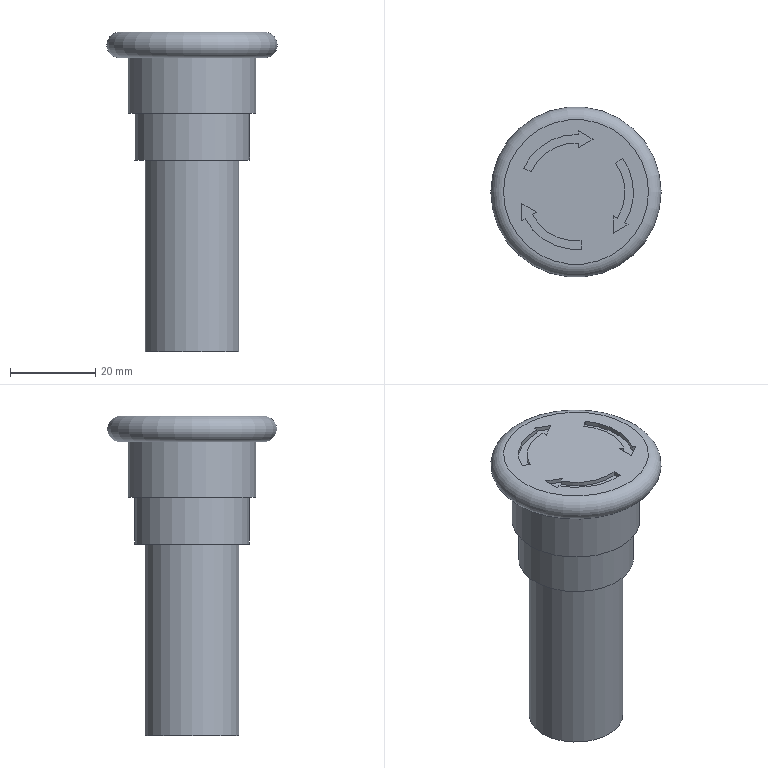Part | NX | 1 solid | 33 faces | box 40 x 40 x 75 mm | volume 39553 mm3 | plane 23 | cylinder 9 | torus 1 | commonest cylinder face diameters 27 x4 23 x3 22 x1 30 x1
STEP:
#1=CARTESIAN_POINT('',(17.,0.,75.));
#2=VERTEX_POINT('',#1);
#3=CARTESIAN_POINT('',(0.,0.,75.));
#4=DIRECTION('',(0.,0.,1.));
#5=DIRECTION('',(1.,0.,0.));
#6=AXIS2_PLACEMENT_3D('',#3,#4,#5);
#7=CIRCLE('',#6,17.);
#8=EDGE_CURVE('',#2,#2,#7,.T.);
#9=ORIENTED_EDGE('',*,*,#8,.F.);
#10=EDGE_LOOP('',(#9));
#11=FACE_BOUND('',#10,.T.);
#12=CARTESIAN_POINT('',(17.,0.,69.));
#13=VERTEX_POINT('',#12);
#14=CARTESIAN_POINT('',(0.,0.,69.));
#15=DIRECTION('',(0.,0.,1.));
#16=DIRECTION('',(1.,0.,0.));
#17=AXIS2_PLACEMENT_3D('',#14,#15,#16);
#18=CIRCLE('',#17,17.);
#19=EDGE_CURVE('',#13,#13,#18,.F.);
#20=ORIENTED_EDGE('',*,*,#19,.F.);
#21=EDGE_LOOP('',(#20));
#22=FACE_BOUND('',#21,.T.);
#23=CARTESIAN_POINT('',(0.,0.,72.));
#24=DIRECTION('',(0.,0.,1.));
#25=DIRECTION('',(1.,0.,0.));
#26=AXIS2_PLACEMENT_3D('',#23,#24,#25);
#27=TOROIDAL_SURFACE('',#26,17.,3.);
#28=ADVANCED_FACE('',(#11,#22),#27,.T.);
#29=CARTESIAN_POINT('',(11.,0.,45.));
#30=VERTEX_POINT('',#29);
#31=CARTESIAN_POINT('',(0.,0.,45.));
#32=DIRECTION('',(0.,0.,1.));
#33=DIRECTION('',(1.,0.,0.));
#34=AXIS2_PLACEMENT_3D('',#31,#32,#33);
#35=CIRCLE('',#34,11.);
#36=EDGE_CURVE('',#30,#30,#35,.T.);
#37=ORIENTED_EDGE('',*,*,#36,.F.);
#38=EDGE_LOOP('',(#37));
#39=FACE_BOUND('',#38,.T.);
#40=CARTESIAN_POINT('',(11.,0.,0.));
#41=VERTEX_POINT('',#40);
#42=CARTESIAN_POINT('',(0.,0.,0.));
#43=DIRECTION('',(0.,0.,1.));
#44=DIRECTION('',(1.,0.,0.));
#45=AXIS2_PLACEMENT_3D('',#42,#43,#44);
#46=CIRCLE('',#45,11.);
#47=EDGE_CURVE('',#41,#41,#46,.T.);
#48=ORIENTED_EDGE('',*,*,#47,.T.);
#49=EDGE_LOOP('',(#48));
#50=FACE_BOUND('',#49,.T.);
#51=CARTESIAN_POINT('',(0.,0.,45.));
#52=DIRECTION('',(0.,0.,-1.));
#53=DIRECTION('',(-1.,0.,0.));
#54=AXIS2_PLACEMENT_3D('',#51,#52,#53);
#55=CYLINDRICAL_SURFACE('',#54,11.);
#56=ADVANCED_FACE('',(#39,#50),#55,.T.);
#57=ORIENTED_EDGE('',*,*,#47,.F.);
#58=EDGE_LOOP('',(#57));
#59=FACE_BOUND('',#58,.T.);
#60=CARTESIAN_POINT('',(0.,0.,0.));
#61=DIRECTION('',(0.,0.,1.));
#62=DIRECTION('',(1.,0.,0.));
#63=AXIS2_PLACEMENT_3D('',#60,#61,#62);
#64=PLANE('',#63);
#65=ADVANCED_FACE('',(#59),#64,.F.);
#66=CARTESIAN_POINT('',(13.5,0.,45.));
#67=VERTEX_POINT('',#66);
#68=CARTESIAN_POINT('',(0.,0.,45.));
#69=DIRECTION('',(0.,0.,1.));
#70=DIRECTION('',(1.,0.,0.));
#71=AXIS2_PLACEMENT_3D('',#68,#69,#70);
#72=CIRCLE('',#71,13.5);
#73=EDGE_CURVE('',#67,#67,#72,.T.);
#74=ORIENTED_EDGE('',*,*,#73,.F.);
#75=EDGE_LOOP('',(#74));
#76=FACE_BOUND('',#75,.T.);
#77=ORIENTED_EDGE('',*,*,#36,.T.);
#78=EDGE_LOOP('',(#77));
#79=FACE_BOUND('',#78,.T.);
#80=CARTESIAN_POINT('',(0.,0.,45.));
#81=DIRECTION('',(0.,0.,1.));
#82=DIRECTION('',(1.,0.,0.));
#83=AXIS2_PLACEMENT_3D('',#80,#81,#82);
#84=PLANE('',#83);
#85=ADVANCED_FACE('',(#76,#79),#84,.F.);
#86=CARTESIAN_POINT('',(13.5,0.,56.));
#87=VERTEX_POINT('',#86);
#88=CARTESIAN_POINT('',(0.,0.,56.));
#89=DIRECTION('',(0.,0.,1.));
#90=DIRECTION('',(1.,0.,0.));
#91=AXIS2_PLACEMENT_3D('',#88,#89,#90);
#92=CIRCLE('',#91,13.5);
#93=EDGE_CURVE('',#87,#87,#92,.T.);
#94=ORIENTED_EDGE('',*,*,#93,.F.);
#95=EDGE_LOOP('',(#94));
#96=FACE_BOUND('',#95,.T.);
#97=ORIENTED_EDGE('',*,*,#73,.T.);
#98=EDGE_LOOP('',(#97));
#99=FACE_BOUND('',#98,.T.);
#100=CARTESIAN_POINT('',(0.,0.,56.));
#101=DIRECTION('',(0.,0.,-1.));
#102=DIRECTION('',(-1.,0.,0.));
#103=AXIS2_PLACEMENT_3D('',#100,#101,#102);
#104=CYLINDRICAL_SURFACE('',#103,13.5);
#105=ADVANCED_FACE('',(#96,#99),#104,.T.);
#106=CARTESIAN_POINT('',(15.,0.,56.));
#107=VERTEX_POINT('',#106);
#108=CARTESIAN_POINT('',(0.,0.,56.));
#109=DIRECTION('',(0.,0.,1.));
#110=DIRECTION('',(1.,0.,0.));
#111=AXIS2_PLACEMENT_3D('',#108,#109,#110);
#112=CIRCLE('',#111,15.);
#113=EDGE_CURVE('',#107,#107,#112,.T.);
#114=ORIENTED_EDGE('',*,*,#113,.F.);
#115=EDGE_LOOP('',(#114));
#116=FACE_BOUND('',#115,.T.);
#117=ORIENTED_EDGE('',*,*,#93,.T.);
#118=EDGE_LOOP('',(#117));
#119=FACE_BOUND('',#118,.T.);
#120=CARTESIAN_POINT('',(0.,0.,56.));
#121=DIRECTION('',(0.,0.,1.));
#122=DIRECTION('',(1.,0.,0.));
#123=AXIS2_PLACEMENT_3D('',#120,#121,#122);
#124=PLANE('',#123);
#125=ADVANCED_FACE('',(#116,#119),#124,.F.);
#126=CARTESIAN_POINT('',(15.,0.,69.));
#127=VERTEX_POINT('',#126);
#128=CARTESIAN_POINT('',(0.,0.,69.));
#129=DIRECTION('',(0.,0.,1.));
#130=DIRECTION('',(1.,0.,0.));
#131=AXIS2_PLACEMENT_3D('',#128,#129,#130);
#132=CIRCLE('',#131,15.);
#133=EDGE_CURVE('',#127,#127,#132,.T.);
#134=ORIENTED_EDGE('',*,*,#133,.F.);
#135=EDGE_LOOP('',(#134));
#136=FACE_BOUND('',#135,.T.);
#137=ORIENTED_EDGE('',*,*,#113,.T.);
#138=EDGE_LOOP('',(#137));
#139=FACE_BOUND('',#138,.T.);
#140=CARTESIAN_POINT('',(0.,0.,69.));
#141=DIRECTION('',(0.,0.,-1.));
#142=DIRECTION('',(-1.,0.,0.));
#143=AXIS2_PLACEMENT_3D('',#140,#141,#142);
#144=CYLINDRICAL_SURFACE('',#143,15.);
#145=ADVANCED_FACE('',(#136,#139),#144,.T.);
#146=ORIENTED_EDGE('',*,*,#19,.T.);
#147=EDGE_LOOP('',(#146));
#148=FACE_BOUND('',#147,.T.);
#149=ORIENTED_EDGE('',*,*,#133,.T.);
#150=EDGE_LOOP('',(#149));
#151=FACE_BOUND('',#150,.T.);
#152=CARTESIAN_POINT('',(0.,0.,69.));
#153=DIRECTION('',(0.,0.,1.));
#154=DIRECTION('',(1.,0.,0.));
#155=AXIS2_PLACEMENT_3D('',#152,#153,#154);
#156=PLANE('',#155);
#157=ADVANCED_FACE('',(#148,#151),#156,.F.);
#158=CARTESIAN_POINT('',(-11.942,-6.295,75.));
#159=VERTEX_POINT('',#158);
#160=CARTESIAN_POINT('',(1.386,-13.429,75.));
#161=VERTEX_POINT('',#160);
#162=CARTESIAN_POINT('',(0.,0.,75.));
#163=DIRECTION('',(0.,0.,1.));
#164=DIRECTION('',(-0.5,0.866,0.));
#165=AXIS2_PLACEMENT_3D('',#162,#163,#164);
#166=CIRCLE('',#165,13.5);
#167=EDGE_CURVE('',#159,#161,#166,.T.);
#168=ORIENTED_EDGE('',*,*,#167,.F.);
#169=CARTESIAN_POINT('',(-12.738,-6.752,75.));
#170=VERTEX_POINT('',#169);
#171=CARTESIAN_POINT('',(-12.738,-6.752,75.));
#172=DIRECTION('',(0.8675,0.4975,0.));
#173=VECTOR('',#172,1000.);
#174=LINE('',#171,#173);
#175=EDGE_CURVE('',#170,#159,#174,.T.);
#176=ORIENTED_EDGE('',*,*,#175,.F.);
#177=CARTESIAN_POINT('',(-12.726,-2.716,75.));
#178=VERTEX_POINT('',#177);
#179=CARTESIAN_POINT('',(-12.726,-2.716,75.));
#180=DIRECTION('',(-0.00291,-1.,0.));
#181=VECTOR('',#180,1000.);
#182=LINE('',#179,#181);
#183=EDGE_CURVE('',#178,#170,#182,.T.);
#184=ORIENTED_EDGE('',*,*,#183,.F.);
#185=CARTESIAN_POINT('',(-9.238,-4.744,75.));
#186=VERTEX_POINT('',#185);
#187=CARTESIAN_POINT('',(-9.238,-4.744,75.));
#188=DIRECTION('',(-0.8646,0.5025,0.));
#189=VECTOR('',#188,1000.);
#190=LINE('',#187,#189);
#191=EDGE_CURVE('',#186,#178,#190,.T.);
#192=ORIENTED_EDGE('',*,*,#191,.F.);
#193=CARTESIAN_POINT('',(-10.206,-5.3,75.));
#194=VERTEX_POINT('',#193);
#195=CARTESIAN_POINT('',(-10.206,-5.3,75.));
#196=DIRECTION('',(0.8675,0.4975,0.));
#197=VECTOR('',#196,1000.);
#198=LINE('',#195,#197);
#199=EDGE_CURVE('',#194,#186,#198,.T.);
#200=ORIENTED_EDGE('',*,*,#199,.F.);
#201=CARTESIAN_POINT('',(1.181,-11.439,75.));
#202=VERTEX_POINT('',#201);
#203=CARTESIAN_POINT('',(0.,0.,75.));
#204=DIRECTION('',(0.,0.,-1.));
#205=DIRECTION('',(-0.5,0.866,0.));
#206=AXIS2_PLACEMENT_3D('',#203,#204,#205);
#207=CIRCLE('',#206,11.5);
#208=EDGE_CURVE('',#202,#194,#207,.T.);
#209=ORIENTED_EDGE('',*,*,#208,.F.);
#210=CARTESIAN_POINT('',(1.386,-13.429,75.));
#211=DIRECTION('',(-0.1027,0.9947,0.));
#212=VECTOR('',#211,1000.);
#213=LINE('',#210,#212);
#214=EDGE_CURVE('',#161,#202,#213,.T.);
#215=ORIENTED_EDGE('',*,*,#214,.F.);
#216=EDGE_LOOP('',(#168,#176,#184,#192,#200,#209,#215));
#217=FACE_BOUND('',#216,.T.);
#218=CARTESIAN_POINT('',(11.423,-7.195,75.));
#219=VERTEX_POINT('',#218);
#220=CARTESIAN_POINT('',(10.937,7.915,75.));
#221=VERTEX_POINT('',#220);
#222=CARTESIAN_POINT('',(0.,0.,75.));
#223=DIRECTION('',(0.,0.,1.));
#224=DIRECTION('',(-0.5,-0.866,0.));
#225=AXIS2_PLACEMENT_3D('',#222,#223,#224);
#226=CIRCLE('',#225,13.5);
#227=EDGE_CURVE('',#219,#221,#226,.T.);
#228=ORIENTED_EDGE('',*,*,#227,.F.);
#229=CARTESIAN_POINT('',(12.216,-7.656,75.));
#230=VERTEX_POINT('',#229);
#231=CARTESIAN_POINT('',(12.216,-7.656,75.));
#232=DIRECTION('',(-0.8646,0.5025,0.));
#233=VECTOR('',#232,1000.);
#234=LINE('',#231,#233);
#235=EDGE_CURVE('',#230,#219,#234,.T.);
#236=ORIENTED_EDGE('',*,*,#235,.F.);
#237=CARTESIAN_POINT('',(8.716,-9.663,75.));
#238=VERTEX_POINT('',#237);
#239=CARTESIAN_POINT('',(8.716,-9.663,75.));
#240=DIRECTION('',(0.8675,0.4975,0.));
#241=VECTOR('',#240,1000.);
#242=LINE('',#239,#241);
#243=EDGE_CURVE('',#238,#230,#242,.T.);
#244=ORIENTED_EDGE('',*,*,#243,.F.);
#245=CARTESIAN_POINT('',(8.727,-5.628,75.));
#246=VERTEX_POINT('',#245);
#247=CARTESIAN_POINT('',(8.727,-5.628,75.));
#248=DIRECTION('',(-0.00291,-1.,0.));
#249=VECTOR('',#248,1000.);
#250=LINE('',#247,#249);
#251=EDGE_CURVE('',#246,#238,#250,.T.);
#252=ORIENTED_EDGE('',*,*,#251,.F.);
#253=CARTESIAN_POINT('',(9.693,-6.189,75.));
#254=VERTEX_POINT('',#253);
#255=CARTESIAN_POINT('',(9.693,-6.189,75.));
#256=DIRECTION('',(-0.8646,0.5025,0.));
#257=VECTOR('',#256,1000.);
#258=LINE('',#255,#257);
#259=EDGE_CURVE('',#254,#246,#258,.T.);
#260=ORIENTED_EDGE('',*,*,#259,.F.);
#261=CARTESIAN_POINT('',(9.316,6.742,75.));
#262=VERTEX_POINT('',#261);
#263=CARTESIAN_POINT('',(0.,0.,75.));
#264=DIRECTION('',(0.,0.,-1.));
#265=DIRECTION('',(-0.5,-0.866,0.));
#266=AXIS2_PLACEMENT_3D('',#263,#264,#265);
#267=CIRCLE('',#266,11.5);
#268=EDGE_CURVE('',#262,#254,#267,.T.);
#269=ORIENTED_EDGE('',*,*,#268,.F.);
#270=CARTESIAN_POINT('',(10.937,7.915,75.));
#271=DIRECTION('',(-0.8101,-0.5863,0.));
#272=VECTOR('',#271,1000.);
#273=LINE('',#270,#272);
#274=EDGE_CURVE('',#221,#262,#273,.T.);
#275=ORIENTED_EDGE('',*,*,#274,.F.);
#276=EDGE_LOOP('',(#228,#236,#244,#252,#260,#269,#275));
#277=FACE_BOUND('',#276,.T.);
#278=CARTESIAN_POINT('',(0.5194,13.49,75.));
#279=VERTEX_POINT('',#278);
#280=CARTESIAN_POINT('',(-12.323,5.514,75.));
#281=VERTEX_POINT('',#280);
#282=CARTESIAN_POINT('',(0.,0.,75.));
#283=DIRECTION('',(0.,0.,1.));
#284=DIRECTION('',(1.,0.,0.));
#285=AXIS2_PLACEMENT_3D('',#282,#283,#284);
#286=CIRCLE('',#285,13.5);
#287=EDGE_CURVE('',#279,#281,#286,.T.);
#288=ORIENTED_EDGE('',*,*,#287,.F.);
#289=CARTESIAN_POINT('',(0.5221,14.407,75.));
#290=VERTEX_POINT('',#289);
#291=CARTESIAN_POINT('',(0.5221,14.407,75.));
#292=DIRECTION('',(-0.00291,-1.,0.));
#293=VECTOR('',#292,1000.);
#294=LINE('',#291,#293);
#295=EDGE_CURVE('',#290,#279,#294,.T.);
#296=ORIENTED_EDGE('',*,*,#295,.F.);
#297=CARTESIAN_POINT('',(4.011,12.38,75.));
#298=VERTEX_POINT('',#297);
#299=CARTESIAN_POINT('',(4.011,12.38,75.));
#300=DIRECTION('',(-0.8646,0.5025,0.));
#301=VECTOR('',#300,1000.);
#302=LINE('',#299,#301);
#303=EDGE_CURVE('',#298,#290,#302,.T.);
#304=ORIENTED_EDGE('',*,*,#303,.F.);
#305=CARTESIAN_POINT('',(0.5103,10.372,75.));
#306=VERTEX_POINT('',#305);
#307=CARTESIAN_POINT('',(0.5103,10.372,75.));
#308=DIRECTION('',(0.8675,0.4975,0.));
#309=VECTOR('',#308,1000.);
#310=LINE('',#307,#309);
#311=EDGE_CURVE('',#306,#298,#310,.T.);
#312=ORIENTED_EDGE('',*,*,#311,.F.);
#313=CARTESIAN_POINT('',(0.5136,11.489,75.));
#314=VERTEX_POINT('',#313);
#315=CARTESIAN_POINT('',(0.5136,11.489,75.));
#316=DIRECTION('',(-0.00291,-1.,0.));
#317=VECTOR('',#316,1000.);
#318=LINE('',#315,#317);
#319=EDGE_CURVE('',#314,#306,#318,.T.);
#320=ORIENTED_EDGE('',*,*,#319,.F.);
#321=CARTESIAN_POINT('',(-10.497,4.697,75.));
#322=VERTEX_POINT('',#321);
#323=CARTESIAN_POINT('',(0.,0.,75.));
#324=DIRECTION('',(0.,0.,-1.));
#325=DIRECTION('',(1.,0.,0.));
#326=AXIS2_PLACEMENT_3D('',#323,#324,#325);
#327=CIRCLE('',#326,11.5);
#328=EDGE_CURVE('',#322,#314,#327,.T.);
#329=ORIENTED_EDGE('',*,*,#328,.F.);
#330=CARTESIAN_POINT('',(-12.323,5.514,75.));
#331=DIRECTION('',(0.9128,-0.4084,0.));
#332=VECTOR('',#331,1000.);
#333=LINE('',#330,#332);
#334=EDGE_CURVE('',#281,#322,#333,.T.);
#335=ORIENTED_EDGE('',*,*,#334,.F.);
#336=EDGE_LOOP('',(#288,#296,#304,#312,#320,#329,#335));
#337=FACE_BOUND('',#336,.T.);
#338=ORIENTED_EDGE('',*,*,#8,.T.);
#339=EDGE_LOOP('',(#338));
#340=FACE_BOUND('',#339,.T.);
#341=CARTESIAN_POINT('',(0.,0.,75.));
#342=DIRECTION('',(0.,0.,1.));
#343=DIRECTION('',(1.,0.,0.));
#344=AXIS2_PLACEMENT_3D('',#341,#342,#343);
#345=PLANE('',#344);
#346=ADVANCED_FACE('',(#217,#277,#337,#340),#345,.T.);
#347=ORIENTED_EDGE('',*,*,#287,.T.);
#348=CARTESIAN_POINT('',(-12.323,5.514,74.));
#349=VERTEX_POINT('',#348);
#350=CARTESIAN_POINT('',(-12.323,5.514,74.));
#351=DIRECTION('',(0.,0.,1.));
#352=VECTOR('',#351,1000.);
#353=LINE('',#350,#352);
#354=EDGE_CURVE('',#349,#281,#353,.T.);
#355=ORIENTED_EDGE('',*,*,#354,.F.);
#356=CARTESIAN_POINT('',(0.5194,13.49,74.));
#357=VERTEX_POINT('',#356);
#358=CARTESIAN_POINT('',(0.,0.,74.));
#359=DIRECTION('',(0.,0.,1.));
#360=DIRECTION('',(1.,0.,0.));
#361=AXIS2_PLACEMENT_3D('',#358,#359,#360);
#362=CIRCLE('',#361,13.5);
#363=EDGE_CURVE('',#357,#349,#362,.T.);
#364=ORIENTED_EDGE('',*,*,#363,.F.);
#365=CARTESIAN_POINT('',(0.5194,13.49,74.));
#366=DIRECTION('',(0.,0.,1.));
#367=VECTOR('',#366,1000.);
#368=LINE('',#365,#367);
#369=EDGE_CURVE('',#357,#279,#368,.T.);
#370=ORIENTED_EDGE('',*,*,#369,.T.);
#371=EDGE_LOOP('',(#347,#355,#364,#370));
#372=FACE_BOUND('',#371,.T.);
#373=CARTESIAN_POINT('',(0.,0.,74.));
#374=DIRECTION('',(0.,0.,1.));
#375=DIRECTION('',(1.,0.,0.));
#376=AXIS2_PLACEMENT_3D('',#373,#374,#375);
#377=CYLINDRICAL_SURFACE('',#376,13.5);
#378=ADVANCED_FACE('',(#372),#377,.F.);
#379=ORIENTED_EDGE('',*,*,#295,.T.);
#380=ORIENTED_EDGE('',*,*,#369,.F.);
#381=CARTESIAN_POINT('',(0.5221,14.407,74.));
#382=VERTEX_POINT('',#381);
#383=CARTESIAN_POINT('',(0.5221,14.407,74.));
#384=DIRECTION('',(-0.00291,-1.,0.));
#385=VECTOR('',#384,1000.);
#386=LINE('',#383,#385);
#387=EDGE_CURVE('',#382,#357,#386,.T.);
#388=ORIENTED_EDGE('',*,*,#387,.F.);
#389=CARTESIAN_POINT('',(0.5221,14.407,74.));
#390=DIRECTION('',(0.,0.,1.));
#391=VECTOR('',#390,1000.);
#392=LINE('',#389,#391);
#393=EDGE_CURVE('',#382,#290,#392,.T.);
#394=ORIENTED_EDGE('',*,*,#393,.T.);
#395=EDGE_LOOP('',(#379,#380,#388,#394));
#396=FACE_BOUND('',#395,.T.);
#397=CARTESIAN_POINT('',(0.5221,14.407,74.));
#398=DIRECTION('',(-1.,0.00291,0.));
#399=DIRECTION('',(-0.00291,-1.,0.));
#400=AXIS2_PLACEMENT_3D('',#397,#398,#399);
#401=PLANE('',#400);
#402=ADVANCED_FACE('',(#396),#401,.F.);
#403=ORIENTED_EDGE('',*,*,#303,.T.);
#404=ORIENTED_EDGE('',*,*,#393,.F.);
#405=CARTESIAN_POINT('',(4.011,12.38,74.));
#406=VERTEX_POINT('',#405);
#407=CARTESIAN_POINT('',(4.011,12.38,74.));
#408=DIRECTION('',(-0.8646,0.5025,0.));
#409=VECTOR('',#408,1000.);
#410=LINE('',#407,#409);
#411=EDGE_CURVE('',#406,#382,#410,.T.);
#412=ORIENTED_EDGE('',*,*,#411,.F.);
#413=CARTESIAN_POINT('',(4.011,12.38,74.));
#414=DIRECTION('',(0.,0.,1.));
#415=VECTOR('',#414,1000.);
#416=LINE('',#413,#415);
#417=EDGE_CURVE('',#406,#298,#416,.T.);
#418=ORIENTED_EDGE('',*,*,#417,.T.);
#419=EDGE_LOOP('',(#403,#404,#412,#418));
#420=FACE_BOUND('',#419,.T.);
#421=CARTESIAN_POINT('',(4.011,12.38,74.));
#422=DIRECTION('',(0.5025,0.8646,0.));
#423=DIRECTION('',(-0.8646,0.5025,0.));
#424=AXIS2_PLACEMENT_3D('',#421,#422,#423);
#425=PLANE('',#424);
#426=ADVANCED_FACE('',(#420),#425,.F.);
#427=ORIENTED_EDGE('',*,*,#311,.T.);
#428=ORIENTED_EDGE('',*,*,#417,.F.);
#429=CARTESIAN_POINT('',(0.5103,10.372,74.));
#430=VERTEX_POINT('',#429);
#431=CARTESIAN_POINT('',(0.5103,10.372,74.));
#432=DIRECTION('',(0.8675,0.4975,0.));
#433=VECTOR('',#432,1000.);
#434=LINE('',#431,#433);
#435=EDGE_CURVE('',#430,#406,#434,.T.);
#436=ORIENTED_EDGE('',*,*,#435,.F.);
#437=CARTESIAN_POINT('',(0.5103,10.372,74.));
#438=DIRECTION('',(0.,0.,1.));
#439=VECTOR('',#438,1000.);
#440=LINE('',#437,#439);
#441=EDGE_CURVE('',#430,#306,#440,.T.);
#442=ORIENTED_EDGE('',*,*,#441,.T.);
#443=EDGE_LOOP('',(#427,#428,#436,#442));
#444=FACE_BOUND('',#443,.T.);
#445=CARTESIAN_POINT('',(0.5103,10.372,74.));
#446=DIRECTION('',(0.4975,-0.8675,0.));
#447=DIRECTION('',(0.8675,0.4975,0.));
#448=AXIS2_PLACEMENT_3D('',#445,#446,#447);
#449=PLANE('',#448);
#450=ADVANCED_FACE('',(#444),#449,.F.);
#451=ORIENTED_EDGE('',*,*,#319,.T.);
#452=ORIENTED_EDGE('',*,*,#441,.F.);
#453=CARTESIAN_POINT('',(0.5136,11.489,74.));
#454=VERTEX_POINT('',#453);
#455=CARTESIAN_POINT('',(0.5136,11.489,74.));
#456=DIRECTION('',(-0.00291,-1.,0.));
#457=VECTOR('',#456,1000.);
#458=LINE('',#455,#457);
#459=EDGE_CURVE('',#454,#430,#458,.T.);
#460=ORIENTED_EDGE('',*,*,#459,.F.);
#461=CARTESIAN_POINT('',(0.5136,11.489,74.));
#462=DIRECTION('',(0.,0.,1.));
#463=VECTOR('',#462,1000.);
#464=LINE('',#461,#463);
#465=EDGE_CURVE('',#454,#314,#464,.T.);
#466=ORIENTED_EDGE('',*,*,#465,.T.);
#467=EDGE_LOOP('',(#451,#452,#460,#466));
#468=FACE_BOUND('',#467,.T.);
#469=CARTESIAN_POINT('',(0.5136,11.489,74.));
#470=DIRECTION('',(-1.,0.00291,0.));
#471=DIRECTION('',(-0.00291,-1.,0.));
#472=AXIS2_PLACEMENT_3D('',#469,#470,#471);
#473=PLANE('',#472);
#474=ADVANCED_FACE('',(#468),#473,.F.);
#475=ORIENTED_EDGE('',*,*,#328,.T.);
#476=ORIENTED_EDGE('',*,*,#465,.F.);
#477=CARTESIAN_POINT('',(-10.497,4.697,74.));
#478=VERTEX_POINT('',#477);
#479=CARTESIAN_POINT('',(0.,0.,74.));
#480=DIRECTION('',(0.,0.,-1.));
#481=DIRECTION('',(1.,0.,0.));
#482=AXIS2_PLACEMENT_3D('',#479,#480,#481);
#483=CIRCLE('',#482,11.5);
#484=EDGE_CURVE('',#478,#454,#483,.T.);
#485=ORIENTED_EDGE('',*,*,#484,.F.);
#486=CARTESIAN_POINT('',(-10.497,4.697,74.));
#487=DIRECTION('',(0.,0.,1.));
#488=VECTOR('',#487,1000.);
#489=LINE('',#486,#488);
#490=EDGE_CURVE('',#478,#322,#489,.T.);
#491=ORIENTED_EDGE('',*,*,#490,.T.);
#492=EDGE_LOOP('',(#475,#476,#485,#491));
#493=FACE_BOUND('',#492,.T.);
#494=CARTESIAN_POINT('',(0.,0.,74.));
#495=DIRECTION('',(0.,0.,1.));
#496=DIRECTION('',(1.,0.,0.));
#497=AXIS2_PLACEMENT_3D('',#494,#495,#496);
#498=CYLINDRICAL_SURFACE('',#497,11.5);
#499=ADVANCED_FACE('',(#493),#498,.T.);
#500=ORIENTED_EDGE('',*,*,#334,.T.);
#501=ORIENTED_EDGE('',*,*,#490,.F.);
#502=CARTESIAN_POINT('',(-12.323,5.514,74.));
#503=DIRECTION('',(0.9128,-0.4084,0.));
#504=VECTOR('',#503,1000.);
#505=LINE('',#502,#504);
#506=EDGE_CURVE('',#349,#478,#505,.T.);
#507=ORIENTED_EDGE('',*,*,#506,.F.);
#508=ORIENTED_EDGE('',*,*,#354,.T.);
#509=EDGE_LOOP('',(#500,#501,#507,#508));
#510=FACE_BOUND('',#509,.T.);
#511=CARTESIAN_POINT('',(-12.323,5.514,74.));
#512=DIRECTION('',(-0.4084,-0.9128,0.));
#513=DIRECTION('',(0.9128,-0.4084,0.));
#514=AXIS2_PLACEMENT_3D('',#511,#512,#513);
#515=PLANE('',#514);
#516=ADVANCED_FACE('',(#510),#515,.F.);
#517=ORIENTED_EDGE('',*,*,#363,.T.);
#518=ORIENTED_EDGE('',*,*,#506,.T.);
#519=ORIENTED_EDGE('',*,*,#484,.T.);
#520=ORIENTED_EDGE('',*,*,#459,.T.);
#521=ORIENTED_EDGE('',*,*,#435,.T.);
#522=ORIENTED_EDGE('',*,*,#411,.T.);
#523=ORIENTED_EDGE('',*,*,#387,.T.);
#524=EDGE_LOOP('',(#517,#518,#519,#520,#521,#522,#523));
#525=FACE_BOUND('',#524,.T.);
#526=CARTESIAN_POINT('',(0.,0.,74.));
#527=DIRECTION('',(0.,0.,1.));
#528=DIRECTION('',(1.,0.,0.));
#529=AXIS2_PLACEMENT_3D('',#526,#527,#528);
#530=PLANE('',#529);
#531=ADVANCED_FACE('',(#525),#530,.T.);
#532=ORIENTED_EDGE('',*,*,#227,.T.);
#533=CARTESIAN_POINT('',(10.937,7.915,74.));
#534=VERTEX_POINT('',#533);
#535=CARTESIAN_POINT('',(10.937,7.915,74.));
#536=DIRECTION('',(0.,0.,1.));
#537=VECTOR('',#536,1000.);
#538=LINE('',#535,#537);
#539=EDGE_CURVE('',#534,#221,#538,.T.);
#540=ORIENTED_EDGE('',*,*,#539,.F.);
#541=CARTESIAN_POINT('',(11.423,-7.195,74.));
#542=VERTEX_POINT('',#541);
#543=CARTESIAN_POINT('',(0.,0.,74.));
#544=DIRECTION('',(0.,0.,1.));
#545=DIRECTION('',(-0.5,-0.866,0.));
#546=AXIS2_PLACEMENT_3D('',#543,#544,#545);
#547=CIRCLE('',#546,13.5);
#548=EDGE_CURVE('',#542,#534,#547,.T.);
#549=ORIENTED_EDGE('',*,*,#548,.F.);
#550=CARTESIAN_POINT('',(11.423,-7.195,74.));
#551=DIRECTION('',(0.,0.,1.));
#552=VECTOR('',#551,1000.);
#553=LINE('',#550,#552);
#554=EDGE_CURVE('',#542,#219,#553,.T.);
#555=ORIENTED_EDGE('',*,*,#554,.T.);
#556=EDGE_LOOP('',(#532,#540,#549,#555));
#557=FACE_BOUND('',#556,.T.);
#558=CARTESIAN_POINT('',(0.,0.,74.));
#559=DIRECTION('',(0.,0.,1.));
#560=DIRECTION('',(1.,0.,0.));
#561=AXIS2_PLACEMENT_3D('',#558,#559,#560);
#562=CYLINDRICAL_SURFACE('',#561,13.5);
#563=ADVANCED_FACE('',(#557),#562,.F.);
#564=ORIENTED_EDGE('',*,*,#235,.T.);
#565=ORIENTED_EDGE('',*,*,#554,.F.);
#566=CARTESIAN_POINT('',(12.216,-7.656,74.));
#567=VERTEX_POINT('',#566);
#568=CARTESIAN_POINT('',(12.216,-7.656,74.));
#569=DIRECTION('',(-0.8646,0.5025,0.));
#570=VECTOR('',#569,1000.);
#571=LINE('',#568,#570);
#572=EDGE_CURVE('',#567,#542,#571,.T.);
#573=ORIENTED_EDGE('',*,*,#572,.F.);
#574=CARTESIAN_POINT('',(12.216,-7.656,74.));
#575=DIRECTION('',(0.,0.,1.));
#576=VECTOR('',#575,1000.);
#577=LINE('',#574,#576);
#578=EDGE_CURVE('',#567,#230,#577,.T.);
#579=ORIENTED_EDGE('',*,*,#578,.T.);
#580=EDGE_LOOP('',(#564,#565,#573,#579));
#581=FACE_BOUND('',#580,.T.);
#582=CARTESIAN_POINT('',(12.216,-7.656,74.));
#583=DIRECTION('',(0.5025,0.8646,0.));
#584=DIRECTION('',(-0.8646,0.5025,0.));
#585=AXIS2_PLACEMENT_3D('',#582,#583,#584);
#586=PLANE('',#585);
#587=ADVANCED_FACE('',(#581),#586,.F.);
#588=ORIENTED_EDGE('',*,*,#243,.T.);
#589=ORIENTED_EDGE('',*,*,#578,.F.);
#590=CARTESIAN_POINT('',(8.716,-9.663,74.));
#591=VERTEX_POINT('',#590);
#592=CARTESIAN_POINT('',(8.716,-9.663,74.));
#593=DIRECTION('',(0.8675,0.4975,0.));
#594=VECTOR('',#593,1000.);
#595=LINE('',#592,#594);
#596=EDGE_CURVE('',#591,#567,#595,.T.);
#597=ORIENTED_EDGE('',*,*,#596,.F.);
#598=CARTESIAN_POINT('',(8.716,-9.663,74.));
#599=DIRECTION('',(0.,0.,1.));
#600=VECTOR('',#599,1000.);
#601=LINE('',#598,#600);
#602=EDGE_CURVE('',#591,#238,#601,.T.);
#603=ORIENTED_EDGE('',*,*,#602,.T.);
#604=EDGE_LOOP('',(#588,#589,#597,#603));
#605=FACE_BOUND('',#604,.T.);
#606=CARTESIAN_POINT('',(8.716,-9.663,74.));
#607=DIRECTION('',(0.4975,-0.8675,0.));
#608=DIRECTION('',(0.8675,0.4975,0.));
#609=AXIS2_PLACEMENT_3D('',#606,#607,#608);
#610=PLANE('',#609);
#611=ADVANCED_FACE('',(#605),#610,.F.);
#612=ORIENTED_EDGE('',*,*,#251,.T.);
#613=ORIENTED_EDGE('',*,*,#602,.F.);
#614=CARTESIAN_POINT('',(8.727,-5.628,74.));
#615=VERTEX_POINT('',#614);
#616=CARTESIAN_POINT('',(8.727,-5.628,74.));
#617=DIRECTION('',(-0.00291,-1.,0.));
#618=VECTOR('',#617,1000.);
#619=LINE('',#616,#618);
#620=EDGE_CURVE('',#615,#591,#619,.T.);
#621=ORIENTED_EDGE('',*,*,#620,.F.);
#622=CARTESIAN_POINT('',(8.727,-5.628,74.));
#623=DIRECTION('',(0.,0.,1.));
#624=VECTOR('',#623,1000.);
#625=LINE('',#622,#624);
#626=EDGE_CURVE('',#615,#246,#625,.T.);
#627=ORIENTED_EDGE('',*,*,#626,.T.);
#628=EDGE_LOOP('',(#612,#613,#621,#627));
#629=FACE_BOUND('',#628,.T.);
#630=CARTESIAN_POINT('',(8.727,-5.628,74.));
#631=DIRECTION('',(-1.,0.00291,0.));
#632=DIRECTION('',(-0.00291,-1.,0.));
#633=AXIS2_PLACEMENT_3D('',#630,#631,#632);
#634=PLANE('',#633);
#635=ADVANCED_FACE('',(#629),#634,.F.);
#636=ORIENTED_EDGE('',*,*,#259,.T.);
#637=ORIENTED_EDGE('',*,*,#626,.F.);
#638=CARTESIAN_POINT('',(9.693,-6.189,74.));
#639=VERTEX_POINT('',#638);
#640=CARTESIAN_POINT('',(9.693,-6.189,74.));
#641=DIRECTION('',(-0.8646,0.5025,0.));
#642=VECTOR('',#641,1000.);
#643=LINE('',#640,#642);
#644=EDGE_CURVE('',#639,#615,#643,.T.);
#645=ORIENTED_EDGE('',*,*,#644,.F.);
#646=CARTESIAN_POINT('',(9.693,-6.189,74.));
#647=DIRECTION('',(0.,0.,1.));
#648=VECTOR('',#647,1000.);
#649=LINE('',#646,#648);
#650=EDGE_CURVE('',#639,#254,#649,.T.);
#651=ORIENTED_EDGE('',*,*,#650,.T.);
#652=EDGE_LOOP('',(#636,#637,#645,#651));
#653=FACE_BOUND('',#652,.T.);
#654=CARTESIAN_POINT('',(9.693,-6.189,74.));
#655=DIRECTION('',(0.5025,0.8646,0.));
#656=DIRECTION('',(-0.8646,0.5025,0.));
#657=AXIS2_PLACEMENT_3D('',#654,#655,#656);
#658=PLANE('',#657);
#659=ADVANCED_FACE('',(#653),#658,.F.);
#660=ORIENTED_EDGE('',*,*,#268,.T.);
#661=ORIENTED_EDGE('',*,*,#650,.F.);
#662=CARTESIAN_POINT('',(9.316,6.742,74.));
#663=VERTEX_POINT('',#662);
#664=CARTESIAN_POINT('',(0.,0.,74.));
#665=DIRECTION('',(0.,0.,-1.));
#666=DIRECTION('',(-0.5,-0.866,0.));
#667=AXIS2_PLACEMENT_3D('',#664,#665,#666);
#668=CIRCLE('',#667,11.5);
#669=EDGE_CURVE('',#663,#639,#668,.T.);
#670=ORIENTED_EDGE('',*,*,#669,.F.);
#671=CARTESIAN_POINT('',(9.316,6.742,74.));
#672=DIRECTION('',(0.,0.,1.));
#673=VECTOR('',#672,1000.);
#674=LINE('',#671,#673);
#675=EDGE_CURVE('',#663,#262,#674,.T.);
#676=ORIENTED_EDGE('',*,*,#675,.T.);
#677=EDGE_LOOP('',(#660,#661,#670,#676));
#678=FACE_BOUND('',#677,.T.);
#679=CARTESIAN_POINT('',(0.,0.,74.));
#680=DIRECTION('',(0.,0.,1.));
#681=DIRECTION('',(1.,0.,0.));
#682=AXIS2_PLACEMENT_3D('',#679,#680,#681);
#683=CYLINDRICAL_SURFACE('',#682,11.5);
#684=ADVANCED_FACE('',(#678),#683,.T.);
#685=ORIENTED_EDGE('',*,*,#274,.T.);
#686=ORIENTED_EDGE('',*,*,#675,.F.);
#687=CARTESIAN_POINT('',(10.937,7.915,74.));
#688=DIRECTION('',(-0.8101,-0.5863,0.));
#689=VECTOR('',#688,1000.);
#690=LINE('',#687,#689);
#691=EDGE_CURVE('',#534,#663,#690,.T.);
#692=ORIENTED_EDGE('',*,*,#691,.F.);
#693=ORIENTED_EDGE('',*,*,#539,.T.);
#694=EDGE_LOOP('',(#685,#686,#692,#693));
#695=FACE_BOUND('',#694,.T.);
#696=CARTESIAN_POINT('',(10.937,7.915,74.));
#697=DIRECTION('',(-0.5863,0.8101,0.));
#698=DIRECTION('',(-0.8101,-0.5863,0.));
#699=AXIS2_PLACEMENT_3D('',#696,#697,#698);
#700=PLANE('',#699);
#701=ADVANCED_FACE('',(#695),#700,.F.);
#702=ORIENTED_EDGE('',*,*,#548,.T.);
#703=ORIENTED_EDGE('',*,*,#691,.T.);
#704=ORIENTED_EDGE('',*,*,#669,.T.);
#705=ORIENTED_EDGE('',*,*,#644,.T.);
#706=ORIENTED_EDGE('',*,*,#620,.T.);
#707=ORIENTED_EDGE('',*,*,#596,.T.);
#708=ORIENTED_EDGE('',*,*,#572,.T.);
#709=EDGE_LOOP('',(#702,#703,#704,#705,#706,#707,#708));
#710=FACE_BOUND('',#709,.T.);
#711=CARTESIAN_POINT('',(0.,0.,74.));
#712=DIRECTION('',(0.,0.,1.));
#713=DIRECTION('',(-0.5,-0.866,0.));
#714=AXIS2_PLACEMENT_3D('',#711,#712,#713);
#715=PLANE('',#714);
#716=ADVANCED_FACE('',(#710),#715,.T.);
#717=ORIENTED_EDGE('',*,*,#167,.T.);
#718=CARTESIAN_POINT('',(1.386,-13.429,74.));
#719=VERTEX_POINT('',#718);
#720=CARTESIAN_POINT('',(1.386,-13.429,74.));
#721=DIRECTION('',(0.,0.,1.));
#722=VECTOR('',#721,1000.);
#723=LINE('',#720,#722);
#724=EDGE_CURVE('',#719,#161,#723,.T.);
#725=ORIENTED_EDGE('',*,*,#724,.F.);
#726=CARTESIAN_POINT('',(-11.942,-6.295,74.));
#727=VERTEX_POINT('',#726);
#728=CARTESIAN_POINT('',(0.,0.,74.));
#729=DIRECTION('',(0.,0.,1.));
#730=DIRECTION('',(-0.5,0.866,0.));
#731=AXIS2_PLACEMENT_3D('',#728,#729,#730);
#732=CIRCLE('',#731,13.5);
#733=EDGE_CURVE('',#727,#719,#732,.T.);
#734=ORIENTED_EDGE('',*,*,#733,.F.);
#735=CARTESIAN_POINT('',(-11.942,-6.295,74.));
#736=DIRECTION('',(0.,0.,1.));
#737=VECTOR('',#736,1000.);
#738=LINE('',#735,#737);
#739=EDGE_CURVE('',#727,#159,#738,.T.);
#740=ORIENTED_EDGE('',*,*,#739,.T.);
#741=EDGE_LOOP('',(#717,#725,#734,#740));
#742=FACE_BOUND('',#741,.T.);
#743=CARTESIAN_POINT('',(0.,0.,74.));
#744=DIRECTION('',(0.,0.,1.));
#745=DIRECTION('',(1.,0.,0.));
#746=AXIS2_PLACEMENT_3D('',#743,#744,#745);
#747=CYLINDRICAL_SURFACE('',#746,13.5);
#748=ADVANCED_FACE('',(#742),#747,.F.);
#749=ORIENTED_EDGE('',*,*,#175,.T.);
#750=ORIENTED_EDGE('',*,*,#739,.F.);
#751=CARTESIAN_POINT('',(-12.738,-6.752,74.));
#752=VERTEX_POINT('',#751);
#753=CARTESIAN_POINT('',(-12.738,-6.752,74.));
#754=DIRECTION('',(0.8675,0.4975,0.));
#755=VECTOR('',#754,1000.);
#756=LINE('',#753,#755);
#757=EDGE_CURVE('',#752,#727,#756,.T.);
#758=ORIENTED_EDGE('',*,*,#757,.F.);
#759=CARTESIAN_POINT('',(-12.738,-6.752,74.));
#760=DIRECTION('',(0.,0.,1.));
#761=VECTOR('',#760,1000.);
#762=LINE('',#759,#761);
#763=EDGE_CURVE('',#752,#170,#762,.T.);
#764=ORIENTED_EDGE('',*,*,#763,.T.);
#765=EDGE_LOOP('',(#749,#750,#758,#764));
#766=FACE_BOUND('',#765,.T.);
#767=CARTESIAN_POINT('',(-12.738,-6.752,74.));
#768=DIRECTION('',(0.4975,-0.8675,0.));
#769=DIRECTION('',(0.8675,0.4975,0.));
#770=AXIS2_PLACEMENT_3D('',#767,#768,#769);
#771=PLANE('',#770);
#772=ADVANCED_FACE('',(#766),#771,.F.);
#773=ORIENTED_EDGE('',*,*,#183,.T.);
#774=ORIENTED_EDGE('',*,*,#763,.F.);
#775=CARTESIAN_POINT('',(-12.726,-2.716,74.));
#776=VERTEX_POINT('',#775);
#777=CARTESIAN_POINT('',(-12.726,-2.716,74.));
#778=DIRECTION('',(-0.00291,-1.,0.));
#779=VECTOR('',#778,1000.);
#780=LINE('',#777,#779);
#781=EDGE_CURVE('',#776,#752,#780,.T.);
#782=ORIENTED_EDGE('',*,*,#781,.F.);
#783=CARTESIAN_POINT('',(-12.726,-2.716,74.));
#784=DIRECTION('',(0.,0.,1.));
#785=VECTOR('',#784,1000.);
#786=LINE('',#783,#785);
#787=EDGE_CURVE('',#776,#178,#786,.T.);
#788=ORIENTED_EDGE('',*,*,#787,.T.);
#789=EDGE_LOOP('',(#773,#774,#782,#788));
#790=FACE_BOUND('',#789,.T.);
#791=CARTESIAN_POINT('',(-12.726,-2.716,74.));
#792=DIRECTION('',(-1.,0.00291,0.));
#793=DIRECTION('',(-0.00291,-1.,0.));
#794=AXIS2_PLACEMENT_3D('',#791,#792,#793);
#795=PLANE('',#794);
#796=ADVANCED_FACE('',(#790),#795,.F.);
#797=ORIENTED_EDGE('',*,*,#191,.T.);
#798=ORIENTED_EDGE('',*,*,#787,.F.);
#799=CARTESIAN_POINT('',(-9.238,-4.744,74.));
#800=VERTEX_POINT('',#799);
#801=CARTESIAN_POINT('',(-9.238,-4.744,74.));
#802=DIRECTION('',(-0.8646,0.5025,0.));
#803=VECTOR('',#802,1000.);
#804=LINE('',#801,#803);
#805=EDGE_CURVE('',#800,#776,#804,.T.);
#806=ORIENTED_EDGE('',*,*,#805,.F.);
#807=CARTESIAN_POINT('',(-9.238,-4.744,74.));
#808=DIRECTION('',(0.,0.,1.));
#809=VECTOR('',#808,1000.);
#810=LINE('',#807,#809);
#811=EDGE_CURVE('',#800,#186,#810,.T.);
#812=ORIENTED_EDGE('',*,*,#811,.T.);
#813=EDGE_LOOP('',(#797,#798,#806,#812));
#814=FACE_BOUND('',#813,.T.);
#815=CARTESIAN_POINT('',(-9.238,-4.744,74.));
#816=DIRECTION('',(0.5025,0.8646,0.));
#817=DIRECTION('',(-0.8646,0.5025,0.));
#818=AXIS2_PLACEMENT_3D('',#815,#816,#817);
#819=PLANE('',#818);
#820=ADVANCED_FACE('',(#814),#819,.F.);
#821=ORIENTED_EDGE('',*,*,#199,.T.);
#822=ORIENTED_EDGE('',*,*,#811,.F.);
#823=CARTESIAN_POINT('',(-10.206,-5.3,74.));
#824=VERTEX_POINT('',#823);
#825=CARTESIAN_POINT('',(-10.206,-5.3,74.));
#826=DIRECTION('',(0.8675,0.4975,0.));
#827=VECTOR('',#826,1000.);
#828=LINE('',#825,#827);
#829=EDGE_CURVE('',#824,#800,#828,.T.);
#830=ORIENTED_EDGE('',*,*,#829,.F.);
#831=CARTESIAN_POINT('',(-10.206,-5.3,74.));
#832=DIRECTION('',(0.,0.,1.));
#833=VECTOR('',#832,1000.);
#834=LINE('',#831,#833);
#835=EDGE_CURVE('',#824,#194,#834,.T.);
#836=ORIENTED_EDGE('',*,*,#835,.T.);
#837=EDGE_LOOP('',(#821,#822,#830,#836));
#838=FACE_BOUND('',#837,.T.);
#839=CARTESIAN_POINT('',(-10.206,-5.3,74.));
#840=DIRECTION('',(0.4975,-0.8675,0.));
#841=DIRECTION('',(0.8675,0.4975,0.));
#842=AXIS2_PLACEMENT_3D('',#839,#840,#841);
#843=PLANE('',#842);
#844=ADVANCED_FACE('',(#838),#843,.F.);
#845=ORIENTED_EDGE('',*,*,#208,.T.);
#846=ORIENTED_EDGE('',*,*,#835,.F.);
#847=CARTESIAN_POINT('',(1.181,-11.439,74.));
#848=VERTEX_POINT('',#847);
#849=CARTESIAN_POINT('',(0.,0.,74.));
#850=DIRECTION('',(0.,0.,-1.));
#851=DIRECTION('',(-0.5,0.866,0.));
#852=AXIS2_PLACEMENT_3D('',#849,#850,#851);
#853=CIRCLE('',#852,11.5);
#854=EDGE_CURVE('',#848,#824,#853,.T.);
#855=ORIENTED_EDGE('',*,*,#854,.F.);
#856=CARTESIAN_POINT('',(1.181,-11.439,74.));
#857=DIRECTION('',(0.,0.,1.));
#858=VECTOR('',#857,1000.);
#859=LINE('',#856,#858);
#860=EDGE_CURVE('',#848,#202,#859,.T.);
#861=ORIENTED_EDGE('',*,*,#860,.T.);
#862=EDGE_LOOP('',(#845,#846,#855,#861));
#863=FACE_BOUND('',#862,.T.);
#864=CARTESIAN_POINT('',(0.,0.,74.));
#865=DIRECTION('',(0.,0.,1.));
#866=DIRECTION('',(1.,0.,0.));
#867=AXIS2_PLACEMENT_3D('',#864,#865,#866);
#868=CYLINDRICAL_SURFACE('',#867,11.5);
#869=ADVANCED_FACE('',(#863),#868,.T.);
#870=ORIENTED_EDGE('',*,*,#214,.T.);
#871=ORIENTED_EDGE('',*,*,#860,.F.);
#872=CARTESIAN_POINT('',(1.386,-13.429,74.));
#873=DIRECTION('',(-0.1027,0.9947,0.));
#874=VECTOR('',#873,1000.);
#875=LINE('',#872,#874);
#876=EDGE_CURVE('',#719,#848,#875,.T.);
#877=ORIENTED_EDGE('',*,*,#876,.F.);
#878=ORIENTED_EDGE('',*,*,#724,.T.);
#879=EDGE_LOOP('',(#870,#871,#877,#878));
#880=FACE_BOUND('',#879,.T.);
#881=CARTESIAN_POINT('',(1.386,-13.429,74.));
#882=DIRECTION('',(0.9947,0.1027,0.));
#883=DIRECTION('',(-0.1027,0.9947,0.));
#884=AXIS2_PLACEMENT_3D('',#881,#882,#883);
#885=PLANE('',#884);
#886=ADVANCED_FACE('',(#880),#885,.F.);
#887=ORIENTED_EDGE('',*,*,#733,.T.);
#888=ORIENTED_EDGE('',*,*,#876,.T.);
#889=ORIENTED_EDGE('',*,*,#854,.T.);
#890=ORIENTED_EDGE('',*,*,#829,.T.);
#891=ORIENTED_EDGE('',*,*,#805,.T.);
#892=ORIENTED_EDGE('',*,*,#781,.T.);
#893=ORIENTED_EDGE('',*,*,#757,.T.);
#894=EDGE_LOOP('',(#887,#888,#889,#890,#891,#892,#893));
#895=FACE_BOUND('',#894,.T.);
#896=CARTESIAN_POINT('',(0.,0.,74.));
#897=DIRECTION('',(0.,0.,1.));
#898=DIRECTION('',(-0.5,0.866,0.));
#899=AXIS2_PLACEMENT_3D('',#896,#897,#898);
#900=PLANE('',#899);
#901=ADVANCED_FACE('',(#895),#900,.T.);
#902=CLOSED_SHELL('',(#28,#56,#65,#85,#105,#125,#145,#157,#346,#378,#402,#426,#450,#474,#499,#516,#531,#563,#587,#611,#635,#659,#684,#701,#716,#748,#772,#796,#820,#844,#869,#886,#901));
#903=MANIFOLD_SOLID_BREP('',#902);
#904=(LENGTH_UNIT()NAMED_UNIT(*)SI_UNIT(.MILLI.,.METRE.));
#905=UNCERTAINTY_MEASURE_WITH_UNIT(LENGTH_MEASURE(0.00001),#904,'','');
#906=(NAMED_UNIT(*)PLANE_ANGLE_UNIT()SI_UNIT($,.RADIAN.));
#907=(NAMED_UNIT(*)SI_UNIT($,.STERADIAN.)SOLID_ANGLE_UNIT());
#908=(GEOMETRIC_REPRESENTATION_CONTEXT(3)GLOBAL_UNCERTAINTY_ASSIGNED_CONTEXT((#905))GLOBAL_UNIT_ASSIGNED_CONTEXT((#904,#906,#907))REPRESENTATION_CONTEXT('',''));
#909=ADVANCED_BREP_SHAPE_REPRESENTATION('',(#903),#908);